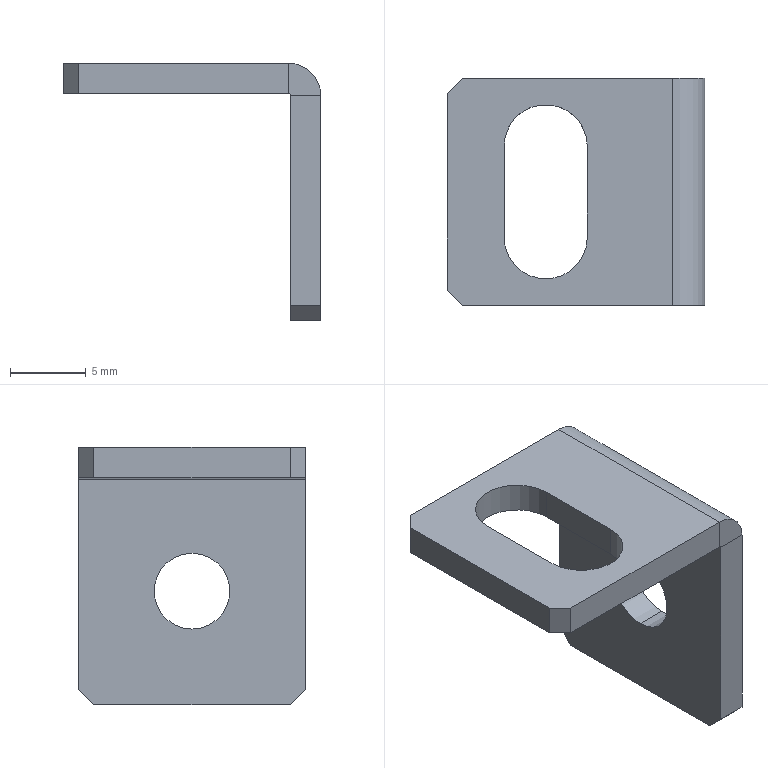Part | STEP file | organic panel mounting plate | 1 solid | 24 faces | box 17 x 15 x 17 mm | volume 789.05 mm3 | plane 18 | cylinder 6 | commonest cylinder face diameters 5 x2 5.5 x2 0.2 x1 4.2 x1